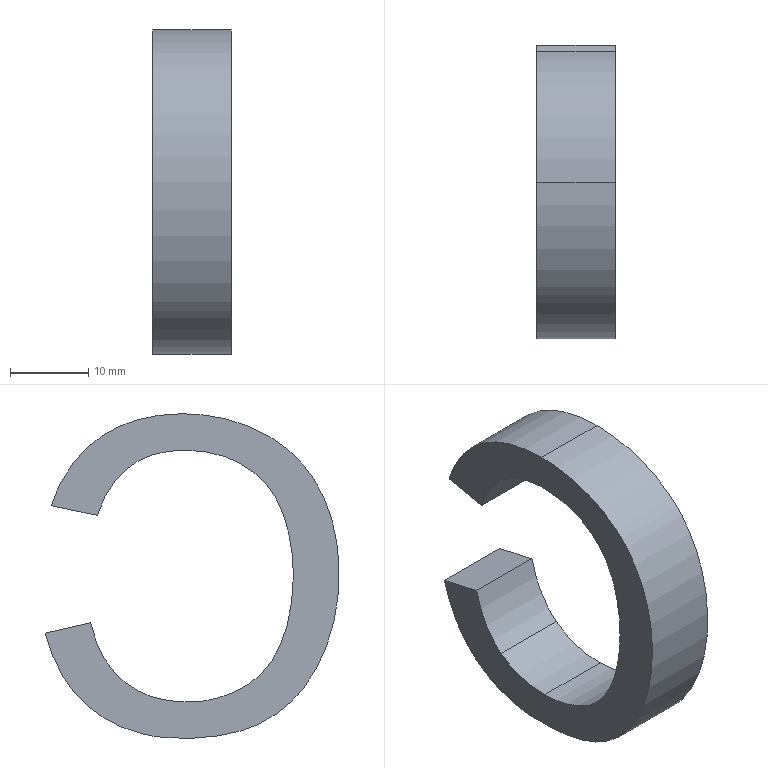Part | NX | features solid 2 | 1 solid | 10 faces | box 10 x 37.644 x 41.56 mm | volume 5171 mm3 | spline 6 | plane 4
STEP:
#1=CARTESIAN_POINT('',(2250.,-497.198,-583.599));
#2=VERTEX_POINT('',#1);
#3=CARTESIAN_POINT('',(2250.,-492.799,-575.973));
#4=VERTEX_POINT('',#3);
#5=CARTESIAN_POINT('',(2250.,-497.198,-583.599));
#6=CARTESIAN_POINT('',(2250.,-495.032,-581.893));
#7=CARTESIAN_POINT('',(2250.,-493.564,-579.369));
#8=CARTESIAN_POINT('',(2250.,-492.799,-575.973));
#9=B_SPLINE_CURVE_WITH_KNOTS('',3,(#5,#6,#7,#8),.UNSPECIFIED.,.F.,.F.,(4,4),(0.,0.03847),.PIECEWISE_BEZIER_KNOTS.);
#10=EDGE_CURVE('',#2,#4,#9,.T.);
#11=ORIENTED_EDGE('',*,*,#10,.F.);
#12=CARTESIAN_POINT('',(2260.,-497.198,-583.599));
#13=VERTEX_POINT('',#12);
#14=CARTESIAN_POINT('',(2260.,-497.198,-583.599));
#15=DIRECTION('',(-1.,0.,0.));
#16=VECTOR('',#15,1000.);
#17=LINE('',#14,#16);
#18=EDGE_CURVE('',#13,#2,#17,.T.);
#19=ORIENTED_EDGE('',*,*,#18,.F.);
#20=CARTESIAN_POINT('',(2260.,-492.799,-575.973));
#21=VERTEX_POINT('',#20);
#22=CARTESIAN_POINT('',(2260.,-497.198,-583.599));
#23=CARTESIAN_POINT('',(2260.,-495.032,-581.893));
#24=CARTESIAN_POINT('',(2260.,-493.564,-579.369));
#25=CARTESIAN_POINT('',(2260.,-492.799,-575.973));
#26=B_SPLINE_CURVE_WITH_KNOTS('',3,(#22,#23,#24,#25),.UNSPECIFIED.,.F.,.F.,(4,4),(0.,0.03847),.PIECEWISE_BEZIER_KNOTS.);
#27=EDGE_CURVE('',#13,#21,#26,.T.);
#28=ORIENTED_EDGE('',*,*,#27,.T.);
#29=CARTESIAN_POINT('',(2260.,-492.799,-575.973));
#30=DIRECTION('',(-1.,0.,0.));
#31=VECTOR('',#30,1000.);
#32=LINE('',#29,#31);
#33=EDGE_CURVE('',#21,#4,#32,.T.);
#34=ORIENTED_EDGE('',*,*,#33,.T.);
#35=EDGE_LOOP('',(#11,#19,#28,#34));
#36=FACE_BOUND('',#35,.T.);
#37=CARTESIAN_POINT('',(2260.,-497.198,-583.599));
#38=CARTESIAN_POINT('',(2250.,-497.198,-583.599));
#39=CARTESIAN_POINT('',(2260.,-495.032,-581.893));
#40=CARTESIAN_POINT('',(2250.,-495.032,-581.893));
#41=CARTESIAN_POINT('',(2260.,-493.564,-579.369));
#42=CARTESIAN_POINT('',(2250.,-493.564,-579.369));
#43=CARTESIAN_POINT('',(2260.,-492.799,-575.973));
#44=CARTESIAN_POINT('',(2250.,-492.799,-575.973));
#45=B_SPLINE_SURFACE_WITH_KNOTS('',3,1,((#37,#38),(#39,#40),(#41,#42),(#43,#44)),.SURF_OF_LINEAR_EXTRUSION.,.F.,.F.,.F.,(4,4),(2,2),(0.,0.03847),(0.,1.),.PIECEWISE_BEZIER_KNOTS.);
#46=ADVANCED_FACE('',(#36),#45,.T.);
#47=CARTESIAN_POINT('',(2250.,-486.956,-577.304));
#48=VERTEX_POINT('',#47);
#49=CARTESIAN_POINT('',(2250.,-492.799,-575.973));
#50=CARTESIAN_POINT('',(2250.,-490.851,-576.417));
#51=CARTESIAN_POINT('',(2250.,-488.903,-576.86));
#52=CARTESIAN_POINT('',(2250.,-486.956,-577.304));
#53=B_SPLINE_CURVE_WITH_KNOTS('',3,(#49,#50,#51,#52),.UNSPECIFIED.,.F.,.F.,(4,4),(0.03847,0.06413),.PIECEWISE_BEZIER_KNOTS.);
#54=EDGE_CURVE('',#4,#48,#53,.T.);
#55=ORIENTED_EDGE('',*,*,#54,.F.);
#56=ORIENTED_EDGE('',*,*,#33,.F.);
#57=CARTESIAN_POINT('',(2260.,-486.956,-577.304));
#58=VERTEX_POINT('',#57);
#59=CARTESIAN_POINT('',(2260.,-492.799,-575.973));
#60=CARTESIAN_POINT('',(2260.,-490.851,-576.417));
#61=CARTESIAN_POINT('',(2260.,-488.903,-576.86));
#62=CARTESIAN_POINT('',(2260.,-486.956,-577.304));
#63=B_SPLINE_CURVE_WITH_KNOTS('',3,(#59,#60,#61,#62),.UNSPECIFIED.,.F.,.F.,(4,4),(0.03847,0.06413),.PIECEWISE_BEZIER_KNOTS.);
#64=EDGE_CURVE('',#21,#58,#63,.T.);
#65=ORIENTED_EDGE('',*,*,#64,.T.);
#66=CARTESIAN_POINT('',(2260.,-486.956,-577.304));
#67=DIRECTION('',(-1.,0.,0.));
#68=VECTOR('',#67,1000.);
#69=LINE('',#66,#68);
#70=EDGE_CURVE('',#58,#48,#69,.T.);
#71=ORIENTED_EDGE('',*,*,#70,.T.);
#72=EDGE_LOOP('',(#55,#56,#65,#71));
#73=FACE_BOUND('',#72,.T.);
#74=CARTESIAN_POINT('',(2260.,-492.799,-575.973));
#75=DIRECTION('',(0.,0.2221,0.975));
#76=DIRECTION('',(0.,-0.975,0.2221));
#77=AXIS2_PLACEMENT_3D('',#74,#75,#76);
#78=PLANE('',#77);
#79=ADVANCED_FACE('',(#73),#78,.T.);
#80=CARTESIAN_POINT('',(2250.,-504.577,-549.22));
#81=VERTEX_POINT('',#80);
#82=CARTESIAN_POINT('',(2250.,-486.956,-577.304));
#83=CARTESIAN_POINT('',(2250.,-488.133,-581.725));
#84=CARTESIAN_POINT('',(2250.,-490.244,-585.075));
#85=CARTESIAN_POINT('',(2250.,-493.321,-587.371));
#86=CARTESIAN_POINT('',(2250.,-496.393,-589.663));
#87=CARTESIAN_POINT('',(2250.,-500.156,-590.78));
#88=CARTESIAN_POINT('',(2250.,-509.166,-590.78));
#89=CARTESIAN_POINT('',(2250.,-512.914,-589.939));
#90=CARTESIAN_POINT('',(2250.,-518.651,-586.398));
#91=CARTESIAN_POINT('',(2250.,-520.822,-583.836));
#92=CARTESIAN_POINT('',(2250.,-523.862,-577.178));
#93=CARTESIAN_POINT('',(2250.,-524.6,-573.572));
#94=CARTESIAN_POINT('',(2250.,-524.6,-565.541));
#95=CARTESIAN_POINT('',(2250.,-523.728,-561.901));
#96=CARTESIAN_POINT('',(2250.,-520.403,-555.646));
#97=CARTESIAN_POINT('',(2250.,-517.977,-553.304));
#98=CARTESIAN_POINT('',(2250.,-511.748,-550.052));
#99=CARTESIAN_POINT('',(2250.,-508.309,-549.25));
#100=CARTESIAN_POINT('',(2250.,-504.577,-549.22));
#101=B_SPLINE_CURVE_WITH_KNOTS('',3,(#82,#83,#84,#85,#86,#87,#88,#89,#90,#91,#92,#93,#94,#95,#96,#97,#98,#99,#100),.UNSPECIFIED.,.F.,.F.,(4,3,2,2,2,2,2,2,4),(0.06413,0.1161,0.1675,0.2204,0.273,0.325,0.3814,0.4374,0.4937),.UNSPECIFIED.);
#102=EDGE_CURVE('',#48,#81,#101,.T.);
#103=ORIENTED_EDGE('',*,*,#102,.F.);
#104=ORIENTED_EDGE('',*,*,#70,.F.);
#105=CARTESIAN_POINT('',(2260.,-504.577,-549.22));
#106=VERTEX_POINT('',#105);
#107=CARTESIAN_POINT('',(2260.,-486.956,-577.304));
#108=CARTESIAN_POINT('',(2260.,-488.133,-581.725));
#109=CARTESIAN_POINT('',(2260.,-490.244,-585.075));
#110=CARTESIAN_POINT('',(2260.,-493.321,-587.371));
#111=CARTESIAN_POINT('',(2260.,-496.393,-589.663));
#112=CARTESIAN_POINT('',(2260.,-500.156,-590.78));
#113=CARTESIAN_POINT('',(2260.,-509.166,-590.78));
#114=CARTESIAN_POINT('',(2260.,-512.914,-589.939));
#115=CARTESIAN_POINT('',(2260.,-518.651,-586.398));
#116=CARTESIAN_POINT('',(2260.,-520.822,-583.836));
#117=CARTESIAN_POINT('',(2260.,-523.862,-577.178));
#118=CARTESIAN_POINT('',(2260.,-524.6,-573.572));
#119=CARTESIAN_POINT('',(2260.,-524.6,-565.541));
#120=CARTESIAN_POINT('',(2260.,-523.728,-561.901));
#121=CARTESIAN_POINT('',(2260.,-520.403,-555.646));
#122=CARTESIAN_POINT('',(2260.,-517.977,-553.304));
#123=CARTESIAN_POINT('',(2260.,-511.748,-550.052));
#124=CARTESIAN_POINT('',(2260.,-508.309,-549.25));
#125=CARTESIAN_POINT('',(2260.,-504.577,-549.22));
#126=B_SPLINE_CURVE_WITH_KNOTS('',3,(#107,#108,#109,#110,#111,#112,#113,#114,#115,#116,#117,#118,#119,#120,#121,#122,#123,#124,#125),.UNSPECIFIED.,.F.,.F.,(4,3,2,2,2,2,2,2,4),(0.06413,0.1161,0.1675,0.2204,0.273,0.325,0.3814,0.4374,0.4937),.UNSPECIFIED.);
#127=EDGE_CURVE('',#58,#106,#126,.T.);
#128=ORIENTED_EDGE('',*,*,#127,.T.);
#129=CARTESIAN_POINT('',(2260.,-504.577,-549.22));
#130=DIRECTION('',(-1.,0.,0.));
#131=VECTOR('',#130,1000.);
#132=LINE('',#129,#131);
#133=EDGE_CURVE('',#106,#81,#132,.T.);
#134=ORIENTED_EDGE('',*,*,#133,.T.);
#135=EDGE_LOOP('',(#103,#104,#128,#134));
#136=FACE_BOUND('',#135,.T.);
#137=CARTESIAN_POINT('',(2260.,-486.956,-577.304));
#138=CARTESIAN_POINT('',(2250.,-486.956,-577.304));
#139=CARTESIAN_POINT('',(2260.,-487.564,-579.587));
#140=CARTESIAN_POINT('',(2250.,-487.564,-579.587));
#141=CARTESIAN_POINT('',(2260.,-489.273,-583.579));
#142=CARTESIAN_POINT('',(2250.,-489.273,-583.579));
#143=CARTESIAN_POINT('',(2260.,-492.7,-587.163));
#144=CARTESIAN_POINT('',(2250.,-492.7,-587.163));
#145=CARTESIAN_POINT('',(2260.,-496.172,-589.175));
#146=CARTESIAN_POINT('',(2250.,-496.172,-589.175));
#147=CARTESIAN_POINT('',(2260.,-499.043,-590.192));
#148=CARTESIAN_POINT('',(2250.,-499.043,-590.192));
#149=CARTESIAN_POINT('',(2260.,-502.172,-590.75));
#150=CARTESIAN_POINT('',(2250.,-502.172,-590.75));
#151=CARTESIAN_POINT('',(2260.,-505.68,-590.821));
#152=CARTESIAN_POINT('',(2250.,-505.68,-590.821));
#153=CARTESIAN_POINT('',(2260.,-508.913,-590.556));
#154=CARTESIAN_POINT('',(2250.,-508.913,-590.556));
#155=CARTESIAN_POINT('',(2260.,-512.779,-589.762));
#156=CARTESIAN_POINT('',(2250.,-512.779,-589.762));
#157=CARTESIAN_POINT('',(2260.,-516.755,-587.864));
#158=CARTESIAN_POINT('',(2250.,-516.755,-587.864));
#159=CARTESIAN_POINT('',(2260.,-520.379,-584.337));
#160=CARTESIAN_POINT('',(2250.,-520.379,-584.337));
#161=CARTESIAN_POINT('',(2260.,-523.033,-579.452));
#162=CARTESIAN_POINT('',(2250.,-523.033,-579.452));
#163=CARTESIAN_POINT('',(2260.,-524.253,-574.873));
#164=CARTESIAN_POINT('',(2250.,-524.253,-574.873));
#165=CARTESIAN_POINT('',(2260.,-524.621,-571.024));
#166=CARTESIAN_POINT('',(2250.,-524.621,-571.024));
#167=CARTESIAN_POINT('',(2260.,-524.595,-567.022));
#168=CARTESIAN_POINT('',(2250.,-524.595,-567.022));
#169=CARTESIAN_POINT('',(2260.,-523.829,-562.55));
#170=CARTESIAN_POINT('',(2250.,-523.829,-562.55));
#171=CARTESIAN_POINT('',(2260.,-521.774,-557.789));
#172=CARTESIAN_POINT('',(2250.,-521.774,-557.789));
#173=CARTESIAN_POINT('',(2260.,-518.688,-554.023));
#174=CARTESIAN_POINT('',(2250.,-518.688,-554.023));
#175=CARTESIAN_POINT('',(2260.,-514.53,-551.28));
#176=CARTESIAN_POINT('',(2250.,-514.53,-551.28));
#177=CARTESIAN_POINT('',(2260.,-509.772,-549.611));
#178=CARTESIAN_POINT('',(2250.,-509.772,-549.611));
#179=CARTESIAN_POINT('',(2260.,-506.356,-549.234));
#180=CARTESIAN_POINT('',(2250.,-506.356,-549.234));
#181=CARTESIAN_POINT('',(2260.,-504.577,-549.22));
#182=CARTESIAN_POINT('',(2250.,-504.577,-549.22));
#183=B_SPLINE_SURFACE_WITH_KNOTS('',3,1,((#137,#138),(#139,#140),(#141,#142),(#143,#144),(#145,#146),(#147,#148),(#149,#150),(#151,#152),(#153,#154),(#155,#156),(#157,#158),(#159,#160),(#161,#162),(#163,#164),(#165,#166),(#167,#168),(#169,#170),(#171,#172),(#173,#174),(#175,#176),(#177,#178),(#179,#180),(#181,#182)),.SURF_OF_LINEAR_EXTRUSION.,.F.,.F.,.F.,(4,1,1,1,1,1,1,1,1,1,1,1,1,1,1,1,1,1,1,1,4),(2,2),(0.06413,0.09098,0.1178,0.1313,0.1447,0.1581,0.1715,0.185,0.1984,0.2252,0.2521,0.2789,0.3058,0.3192,0.3326,0.3595,0.3863,0.4132,0.44,0.4669,0.4937),(0.,1.),.UNSPECIFIED.);
#184=ADVANCED_FACE('',(#136),#183,.T.);
#185=CARTESIAN_POINT('',(2250.,-487.782,-560.998));
#186=VERTEX_POINT('',#185);
#187=CARTESIAN_POINT('',(2250.,-504.577,-549.22));
#188=CARTESIAN_POINT('',(2250.,-500.309,-549.25));
#189=CARTESIAN_POINT('',(2250.,-496.73,-550.291));
#190=CARTESIAN_POINT('',(2250.,-490.944,-554.415));
#191=CARTESIAN_POINT('',(2250.,-488.944,-557.312));
#192=CARTESIAN_POINT('',(2250.,-487.782,-560.998));
#193=B_SPLINE_CURVE_WITH_KNOTS('',3,(#187,#188,#189,#190,#191,#192),.UNSPECIFIED.,.F.,.F.,(4,2,4),(0.4937,0.5474,0.6018),.UNSPECIFIED.);
#194=EDGE_CURVE('',#81,#186,#193,.T.);
#195=ORIENTED_EDGE('',*,*,#194,.F.);
#196=ORIENTED_EDGE('',*,*,#133,.F.);
#197=CARTESIAN_POINT('',(2260.,-487.782,-560.998));
#198=VERTEX_POINT('',#197);
#199=CARTESIAN_POINT('',(2260.,-504.577,-549.22));
#200=CARTESIAN_POINT('',(2260.,-500.309,-549.25));
#201=CARTESIAN_POINT('',(2260.,-496.73,-550.291));
#202=CARTESIAN_POINT('',(2260.,-490.944,-554.415));
#203=CARTESIAN_POINT('',(2260.,-488.944,-557.312));
#204=CARTESIAN_POINT('',(2260.,-487.782,-560.998));
#205=B_SPLINE_CURVE_WITH_KNOTS('',3,(#199,#200,#201,#202,#203,#204),.UNSPECIFIED.,.F.,.F.,(4,2,4),(0.4937,0.5474,0.6018),.UNSPECIFIED.);
#206=EDGE_CURVE('',#106,#198,#205,.T.);
#207=ORIENTED_EDGE('',*,*,#206,.T.);
#208=CARTESIAN_POINT('',(2260.,-487.782,-560.998));
#209=DIRECTION('',(-1.,0.,0.));
#210=VECTOR('',#209,1000.);
#211=LINE('',#208,#210);
#212=EDGE_CURVE('',#198,#186,#211,.T.);
#213=ORIENTED_EDGE('',*,*,#212,.T.);
#214=EDGE_LOOP('',(#195,#196,#207,#213));
#215=FACE_BOUND('',#214,.T.);
#216=CARTESIAN_POINT('',(2260.,-504.577,-549.22));
#217=CARTESIAN_POINT('',(2250.,-504.577,-549.22));
#218=CARTESIAN_POINT('',(2260.,-502.43,-549.235));
#219=CARTESIAN_POINT('',(2250.,-502.43,-549.235));
#220=CARTESIAN_POINT('',(2260.,-498.492,-549.769));
#221=CARTESIAN_POINT('',(2250.,-498.492,-549.769));
#222=CARTESIAN_POINT('',(2260.,-493.6,-552.149));
#223=CARTESIAN_POINT('',(2250.,-493.6,-552.149));
#224=CARTESIAN_POINT('',(2260.,-489.922,-555.899));
#225=CARTESIAN_POINT('',(2250.,-489.922,-555.899));
#226=CARTESIAN_POINT('',(2260.,-488.359,-559.166));
#227=CARTESIAN_POINT('',(2250.,-488.359,-559.166));
#228=CARTESIAN_POINT('',(2260.,-487.782,-560.998));
#229=CARTESIAN_POINT('',(2250.,-487.782,-560.998));
#230=B_SPLINE_SURFACE_WITH_KNOTS('',3,1,((#216,#217),(#218,#219),(#220,#221),(#222,#223),(#224,#225),(#226,#227),(#228,#229)),.SURF_OF_LINEAR_EXTRUSION.,.F.,.F.,.F.,(4,1,1,1,4),(2,2),(0.4937,0.5207,0.5478,0.5748,0.6018),(0.,1.),.UNSPECIFIED.);
#231=ADVANCED_FACE('',(#215),#230,.T.);
#232=CARTESIAN_POINT('',(2250.,-493.64,-562.237));
#233=VERTEX_POINT('',#232);
#234=CARTESIAN_POINT('',(2250.,-487.782,-560.998));
#235=CARTESIAN_POINT('',(2250.,-489.734,-561.411));
#236=CARTESIAN_POINT('',(2250.,-491.687,-561.824));
#237=CARTESIAN_POINT('',(2250.,-493.64,-562.237));
#238=B_SPLINE_CURVE_WITH_KNOTS('',3,(#234,#235,#236,#237),.UNSPECIFIED.,.F.,.F.,(4,4),(0.6018,0.6302),.PIECEWISE_BEZIER_KNOTS.);
#239=EDGE_CURVE('',#186,#233,#238,.T.);
#240=ORIENTED_EDGE('',*,*,#239,.F.);
#241=ORIENTED_EDGE('',*,*,#212,.F.);
#242=CARTESIAN_POINT('',(2260.,-493.64,-562.237));
#243=VERTEX_POINT('',#242);
#244=CARTESIAN_POINT('',(2260.,-487.782,-560.998));
#245=CARTESIAN_POINT('',(2260.,-489.734,-561.411));
#246=CARTESIAN_POINT('',(2260.,-491.687,-561.824));
#247=CARTESIAN_POINT('',(2260.,-493.64,-562.237));
#248=B_SPLINE_CURVE_WITH_KNOTS('',3,(#244,#245,#246,#247),.UNSPECIFIED.,.F.,.F.,(4,4),(0.6018,0.6302),.PIECEWISE_BEZIER_KNOTS.);
#249=EDGE_CURVE('',#198,#243,#248,.T.);
#250=ORIENTED_EDGE('',*,*,#249,.T.);
#251=CARTESIAN_POINT('',(2260.,-493.64,-562.237));
#252=DIRECTION('',(-1.,0.,0.));
#253=VECTOR('',#252,1000.);
#254=LINE('',#251,#253);
#255=EDGE_CURVE('',#243,#233,#254,.T.);
#256=ORIENTED_EDGE('',*,*,#255,.T.);
#257=EDGE_LOOP('',(#240,#241,#250,#256));
#258=FACE_BOUND('',#257,.T.);
#259=CARTESIAN_POINT('',(2260.,-487.782,-560.998));
#260=DIRECTION('',(0.,0.2069,-0.9784));
#261=DIRECTION('',(0.,0.9784,0.2069));
#262=AXIS2_PLACEMENT_3D('',#259,#260,#261);
#263=PLANE('',#262);
#264=ADVANCED_FACE('',(#258),#263,.T.);
#265=CARTESIAN_POINT('',(2250.,-504.837,-553.885));
#266=VERTEX_POINT('',#265);
#267=CARTESIAN_POINT('',(2250.,-493.64,-562.237));
#268=CARTESIAN_POINT('',(2250.,-494.604,-559.346));
#269=CARTESIAN_POINT('',(2250.,-496.026,-557.235));
#270=CARTESIAN_POINT('',(2250.,-499.711,-554.586));
#271=CARTESIAN_POINT('',(2250.,-502.038,-553.916));
#272=CARTESIAN_POINT('',(2250.,-504.837,-553.885));
#273=B_SPLINE_CURVE_WITH_KNOTS('',3,(#267,#268,#269,#270,#271,#272),.UNSPECIFIED.,.F.,.F.,(4,2,4),(0.6302,0.6671,0.7036),.UNSPECIFIED.);
#274=EDGE_CURVE('',#233,#266,#273,.T.);
#275=ORIENTED_EDGE('',*,*,#274,.F.);
#276=ORIENTED_EDGE('',*,*,#255,.F.);
#277=CARTESIAN_POINT('',(2260.,-504.837,-553.885));
#278=VERTEX_POINT('',#277);
#279=CARTESIAN_POINT('',(2260.,-493.64,-562.237));
#280=CARTESIAN_POINT('',(2260.,-494.604,-559.346));
#281=CARTESIAN_POINT('',(2260.,-496.026,-557.235));
#282=CARTESIAN_POINT('',(2260.,-499.711,-554.586));
#283=CARTESIAN_POINT('',(2260.,-502.038,-553.916));
#284=CARTESIAN_POINT('',(2260.,-504.837,-553.885));
#285=B_SPLINE_CURVE_WITH_KNOTS('',3,(#279,#280,#281,#282,#283,#284),.UNSPECIFIED.,.F.,.F.,(4,2,4),(0.6302,0.6671,0.7036),.UNSPECIFIED.);
#286=EDGE_CURVE('',#243,#278,#285,.T.);
#287=ORIENTED_EDGE('',*,*,#286,.T.);
#288=CARTESIAN_POINT('',(2260.,-504.837,-553.885));
#289=DIRECTION('',(-1.,0.,0.));
#290=VECTOR('',#289,1000.);
#291=LINE('',#288,#290);
#292=EDGE_CURVE('',#278,#266,#291,.T.);
#293=ORIENTED_EDGE('',*,*,#292,.T.);
#294=EDGE_LOOP('',(#275,#276,#287,#293));
#295=FACE_BOUND('',#294,.T.);
#296=CARTESIAN_POINT('',(2260.,-493.64,-562.237));
#297=CARTESIAN_POINT('',(2250.,-493.64,-562.237));
#298=CARTESIAN_POINT('',(2260.,-495.558,-556.482));
#299=CARTESIAN_POINT('',(2250.,-495.558,-556.482));
#300=CARTESIAN_POINT('',(2260.,-499.212,-553.947));
#301=CARTESIAN_POINT('',(2250.,-499.212,-553.947));
#302=CARTESIAN_POINT('',(2260.,-504.837,-553.885));
#303=CARTESIAN_POINT('',(2250.,-504.837,-553.885));
#304=B_SPLINE_SURFACE_WITH_KNOTS('',3,1,((#296,#297),(#298,#299),(#300,#301),(#302,#303)),.SURF_OF_LINEAR_EXTRUSION.,.F.,.F.,.F.,(4,4),(2,2),(0.6302,0.7036),(0.,1.),.PIECEWISE_BEZIER_KNOTS.);
#305=ADVANCED_FACE('',(#295),#304,.T.);
#306=CARTESIAN_POINT('',(2250.,-505.143,-586.115));
#307=VERTEX_POINT('',#306);
#308=CARTESIAN_POINT('',(2250.,-504.837,-553.885));
#309=CARTESIAN_POINT('',(2250.,-508.019,-553.916));
#310=CARTESIAN_POINT('',(2250.,-510.711,-554.665));
#311=CARTESIAN_POINT('',(2250.,-512.871,-556.136));
#312=CARTESIAN_POINT('',(2250.,-515.024,-557.602));
#313=CARTESIAN_POINT('',(2250.,-516.539,-559.56));
#314=CARTESIAN_POINT('',(2250.,-518.311,-564.511));
#315=CARTESIAN_POINT('',(2250.,-518.741,-567.071));
#316=CARTESIAN_POINT('',(2250.,-518.741,-573.113));
#317=CARTESIAN_POINT('',(2250.,-518.221,-576.08));
#318=CARTESIAN_POINT('',(2250.,-516.107,-581.136));
#319=CARTESIAN_POINT('',(2250.,-514.504,-583.04));
#320=CARTESIAN_POINT('',(2250.,-510.104,-585.515));
#321=CARTESIAN_POINT('',(2250.,-507.713,-586.145));
#322=CARTESIAN_POINT('',(2250.,-505.143,-586.115));
#323=B_SPLINE_CURVE_WITH_KNOTS('',3,(#308,#309,#310,#311,#312,#313,#314,#315,#316,#317,#318,#319,#320,#321,#322),.UNSPECIFIED.,.F.,.F.,(4,3,2,2,2,2,4),(0.7036,0.744,0.7802,0.8163,0.8636,0.911,0.9584),.UNSPECIFIED.);
#324=EDGE_CURVE('',#266,#307,#323,.T.);
#325=ORIENTED_EDGE('',*,*,#324,.F.);
#326=ORIENTED_EDGE('',*,*,#292,.F.);
#327=CARTESIAN_POINT('',(2260.,-505.143,-586.115));
#328=VERTEX_POINT('',#327);
#329=CARTESIAN_POINT('',(2260.,-504.837,-553.885));
#330=CARTESIAN_POINT('',(2260.,-508.019,-553.916));
#331=CARTESIAN_POINT('',(2260.,-510.711,-554.665));
#332=CARTESIAN_POINT('',(2260.,-512.871,-556.136));
#333=CARTESIAN_POINT('',(2260.,-515.024,-557.602));
#334=CARTESIAN_POINT('',(2260.,-516.539,-559.56));
#335=CARTESIAN_POINT('',(2260.,-518.311,-564.511));
#336=CARTESIAN_POINT('',(2260.,-518.741,-567.071));
#337=CARTESIAN_POINT('',(2260.,-518.741,-573.113));
#338=CARTESIAN_POINT('',(2260.,-518.221,-576.08));
#339=CARTESIAN_POINT('',(2260.,-516.107,-581.136));
#340=CARTESIAN_POINT('',(2260.,-514.504,-583.04));
#341=CARTESIAN_POINT('',(2260.,-510.104,-585.515));
#342=CARTESIAN_POINT('',(2260.,-507.713,-586.145));
#343=CARTESIAN_POINT('',(2260.,-505.143,-586.115));
#344=B_SPLINE_CURVE_WITH_KNOTS('',3,(#329,#330,#331,#332,#333,#334,#335,#336,#337,#338,#339,#340,#341,#342,#343),.UNSPECIFIED.,.F.,.F.,(4,3,2,2,2,2,4),(0.7036,0.744,0.7802,0.8163,0.8636,0.911,0.9584),.UNSPECIFIED.);
#345=EDGE_CURVE('',#278,#328,#344,.T.);
#346=ORIENTED_EDGE('',*,*,#345,.T.);
#347=CARTESIAN_POINT('',(2260.,-505.143,-586.115));
#348=DIRECTION('',(-1.,0.,0.));
#349=VECTOR('',#348,1000.);
#350=LINE('',#347,#349);
#351=EDGE_CURVE('',#328,#307,#350,.T.);
#352=ORIENTED_EDGE('',*,*,#351,.T.);
#353=EDGE_LOOP('',(#325,#326,#346,#352));
#354=FACE_BOUND('',#353,.T.);
#355=CARTESIAN_POINT('',(2260.,-504.837,-553.885));
#356=CARTESIAN_POINT('',(2250.,-504.837,-553.885));
#357=CARTESIAN_POINT('',(2260.,-506.092,-553.897));
#358=CARTESIAN_POINT('',(2250.,-506.092,-553.897));
#359=CARTESIAN_POINT('',(2260.,-508.442,-554.14));
#360=CARTESIAN_POINT('',(2250.,-508.442,-554.14));
#361=CARTESIAN_POINT('',(2260.,-511.019,-555.028));
#362=CARTESIAN_POINT('',(2250.,-511.019,-555.028));
#363=CARTESIAN_POINT('',(2260.,-512.767,-556.022));
#364=CARTESIAN_POINT('',(2250.,-512.767,-556.022));
#365=CARTESIAN_POINT('',(2260.,-514.606,-557.428));
#366=CARTESIAN_POINT('',(2250.,-514.606,-557.428));
#367=CARTESIAN_POINT('',(2260.,-516.363,-559.47));
#368=CARTESIAN_POINT('',(2250.,-516.363,-559.47));
#369=CARTESIAN_POINT('',(2260.,-517.737,-562.635));
#370=CARTESIAN_POINT('',(2250.,-517.737,-562.635));
#371=CARTESIAN_POINT('',(2260.,-518.534,-565.987));
#372=CARTESIAN_POINT('',(2250.,-518.534,-565.987));
#373=CARTESIAN_POINT('',(2260.,-518.815,-569.435));
#374=CARTESIAN_POINT('',(2250.,-518.815,-569.435));
#375=CARTESIAN_POINT('',(2260.,-518.592,-573.928));
#376=CARTESIAN_POINT('',(2250.,-518.592,-573.928));
#377=CARTESIAN_POINT('',(2260.,-517.457,-578.715));
#378=CARTESIAN_POINT('',(2250.,-517.457,-578.715));
#379=CARTESIAN_POINT('',(2260.,-514.649,-583.072));
#380=CARTESIAN_POINT('',(2250.,-514.649,-583.072));
#381=CARTESIAN_POINT('',(2260.,-510.153,-585.572));
#382=CARTESIAN_POINT('',(2250.,-510.153,-585.572));
#383=CARTESIAN_POINT('',(2260.,-506.872,-586.135));
#384=CARTESIAN_POINT('',(2250.,-506.872,-586.135));
#385=CARTESIAN_POINT('',(2260.,-505.143,-586.115));
#386=CARTESIAN_POINT('',(2250.,-505.143,-586.115));
#387=B_SPLINE_SURFACE_WITH_KNOTS('',3,1,((#355,#356),(#357,#358),(#359,#360),(#361,#362),(#363,#364),(#365,#366),(#367,#368),(#369,#370),(#371,#372),(#373,#374),(#375,#376),(#377,#378),(#379,#380),(#381,#382),(#383,#384),(#385,#386)),.SURF_OF_LINEAR_EXTRUSION.,.F.,.F.,.F.,(4,1,1,1,1,1,1,1,1,1,1,1,1,4),(2,2),(0.7036,0.7195,0.7355,0.7434,0.7514,0.7673,0.7832,0.7991,0.8151,0.831,0.8628,0.8947,0.9265,0.9584),(0.,1.),.UNSPECIFIED.);
#388=ADVANCED_FACE('',(#354),#387,.T.);
#389=CARTESIAN_POINT('',(2250.,-505.143,-586.115));
#390=CARTESIAN_POINT('',(2250.,-502.007,-586.145));
#391=CARTESIAN_POINT('',(2250.,-499.361,-585.304));
#392=CARTESIAN_POINT('',(2250.,-497.198,-583.599));
#393=B_SPLINE_CURVE_WITH_KNOTS('',3,(#389,#390,#391,#392),.UNSPECIFIED.,.F.,.F.,(4,4),(0.9584,1.),.PIECEWISE_BEZIER_KNOTS.);
#394=EDGE_CURVE('',#307,#2,#393,.T.);
#395=ORIENTED_EDGE('',*,*,#394,.F.);
#396=ORIENTED_EDGE('',*,*,#351,.F.);
#397=CARTESIAN_POINT('',(2260.,-505.143,-586.115));
#398=CARTESIAN_POINT('',(2260.,-502.007,-586.145));
#399=CARTESIAN_POINT('',(2260.,-499.361,-585.304));
#400=CARTESIAN_POINT('',(2260.,-497.198,-583.599));
#401=B_SPLINE_CURVE_WITH_KNOTS('',3,(#397,#398,#399,#400),.UNSPECIFIED.,.F.,.F.,(4,4),(0.9584,1.),.PIECEWISE_BEZIER_KNOTS.);
#402=EDGE_CURVE('',#328,#13,#401,.T.);
#403=ORIENTED_EDGE('',*,*,#402,.T.);
#404=ORIENTED_EDGE('',*,*,#18,.T.);
#405=EDGE_LOOP('',(#395,#396,#403,#404));
#406=FACE_BOUND('',#405,.T.);
#407=CARTESIAN_POINT('',(2260.,-505.143,-586.115));
#408=CARTESIAN_POINT('',(2250.,-505.143,-586.115));
#409=CARTESIAN_POINT('',(2260.,-502.007,-586.145));
#410=CARTESIAN_POINT('',(2250.,-502.007,-586.145));
#411=CARTESIAN_POINT('',(2260.,-499.361,-585.304));
#412=CARTESIAN_POINT('',(2250.,-499.361,-585.304));
#413=CARTESIAN_POINT('',(2260.,-497.198,-583.599));
#414=CARTESIAN_POINT('',(2250.,-497.198,-583.599));
#415=B_SPLINE_SURFACE_WITH_KNOTS('',3,1,((#407,#408),(#409,#410),(#411,#412),(#413,#414)),.SURF_OF_LINEAR_EXTRUSION.,.F.,.F.,.F.,(4,4),(2,2),(0.9584,1.),(0.,1.),.PIECEWISE_BEZIER_KNOTS.);
#416=ADVANCED_FACE('',(#406),#415,.T.);
#417=ORIENTED_EDGE('',*,*,#27,.F.);
#418=ORIENTED_EDGE('',*,*,#402,.F.);
#419=ORIENTED_EDGE('',*,*,#345,.F.);
#420=ORIENTED_EDGE('',*,*,#286,.F.);
#421=ORIENTED_EDGE('',*,*,#249,.F.);
#422=ORIENTED_EDGE('',*,*,#206,.F.);
#423=ORIENTED_EDGE('',*,*,#127,.F.);
#424=ORIENTED_EDGE('',*,*,#64,.F.);
#425=EDGE_LOOP('',(#417,#418,#419,#420,#421,#422,#423,#424));
#426=FACE_BOUND('',#425,.T.);
#427=CARTESIAN_POINT('',(2260.,-494.473,-580.42));
#428=DIRECTION('',(-1.,0.,0.));
#429=DIRECTION('',(0.,-1.,0.));
#430=AXIS2_PLACEMENT_3D('',#427,#428,#429);
#431=PLANE('',#430);
#432=ADVANCED_FACE('',(#426),#431,.F.);
#433=ORIENTED_EDGE('',*,*,#10,.T.);
#434=ORIENTED_EDGE('',*,*,#54,.T.);
#435=ORIENTED_EDGE('',*,*,#102,.T.);
#436=ORIENTED_EDGE('',*,*,#194,.T.);
#437=ORIENTED_EDGE('',*,*,#239,.T.);
#438=ORIENTED_EDGE('',*,*,#274,.T.);
#439=ORIENTED_EDGE('',*,*,#324,.T.);
#440=ORIENTED_EDGE('',*,*,#394,.T.);
#441=EDGE_LOOP('',(#433,#434,#435,#436,#437,#438,#439,#440));
#442=FACE_BOUND('',#441,.T.);
#443=CARTESIAN_POINT('',(2250.,-494.473,-580.42));
#444=DIRECTION('',(-1.,0.,0.));
#445=DIRECTION('',(0.,-1.,0.));
#446=AXIS2_PLACEMENT_3D('',#443,#444,#445);
#447=PLANE('',#446);
#448=ADVANCED_FACE('',(#442),#447,.T.);
#449=CLOSED_SHELL('',(#46,#79,#184,#231,#264,#305,#388,#416,#432,#448));
#450=MANIFOLD_SOLID_BREP('',#449);
#451=(LENGTH_UNIT()NAMED_UNIT(*)SI_UNIT(.MILLI.,.METRE.));
#452=UNCERTAINTY_MEASURE_WITH_UNIT(LENGTH_MEASURE(0.0508),#451,'','');
#453=(NAMED_UNIT(*)PLANE_ANGLE_UNIT()SI_UNIT($,.RADIAN.));
#454=(NAMED_UNIT(*)SI_UNIT($,.STERADIAN.)SOLID_ANGLE_UNIT());
#455=(GEOMETRIC_REPRESENTATION_CONTEXT(3)GLOBAL_UNCERTAINTY_ASSIGNED_CONTEXT((#452))GLOBAL_UNIT_ASSIGNED_CONTEXT((#451,#453,#454))REPRESENTATION_CONTEXT('',''));
#456=ADVANCED_BREP_SHAPE_REPRESENTATION('',(#450),#455);